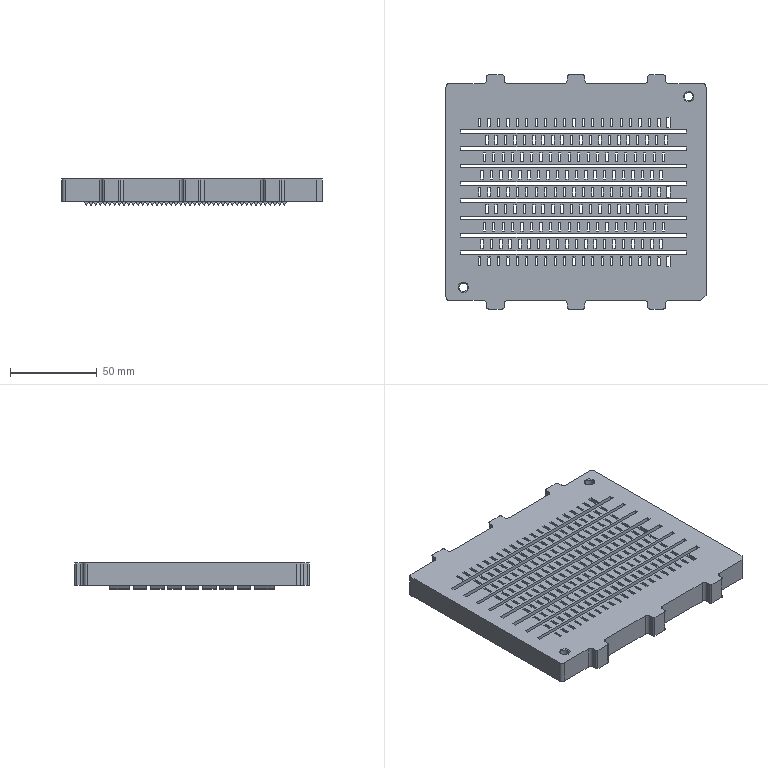Part | STEP file | 1 solid | 2555 faces | box 150 x 135 x 15 mm | volume 212258 mm3 | plane 1574 | cylinder 977 | cone 4 | commonest cylinder face diameters 0.68 x490 0.72 x458 4 x15 2 x12 5 x2